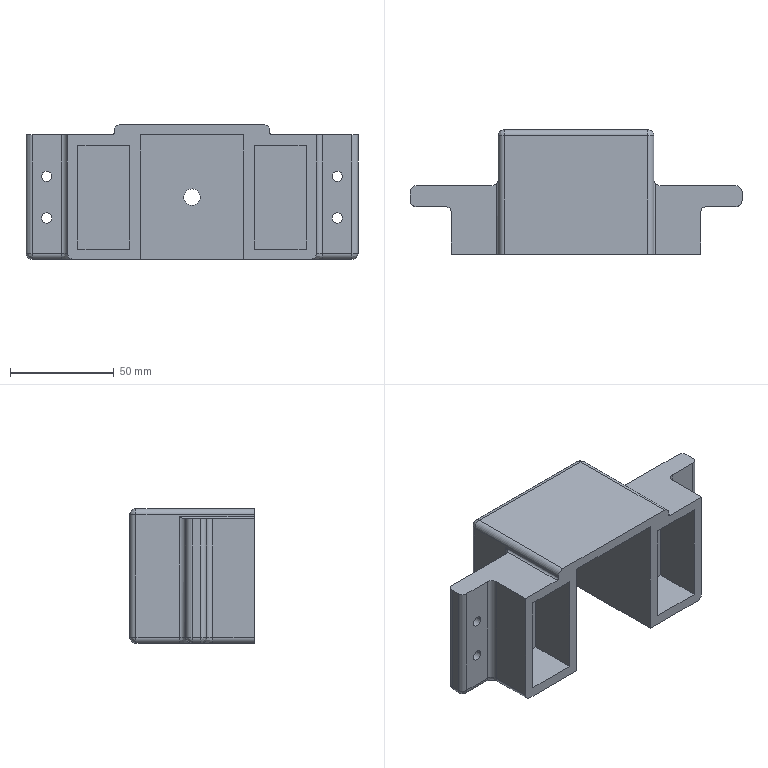Part | SolidWorks | features BaseBody 1 | 1 solid | 78 faces | box 160 x 60 x 65 mm | volume 180425 mm3 | cylinder 34 | plane 30 | spline 12 | cone 2 | commonest cylinder face diameters 6 x24 5 x8 2 x2